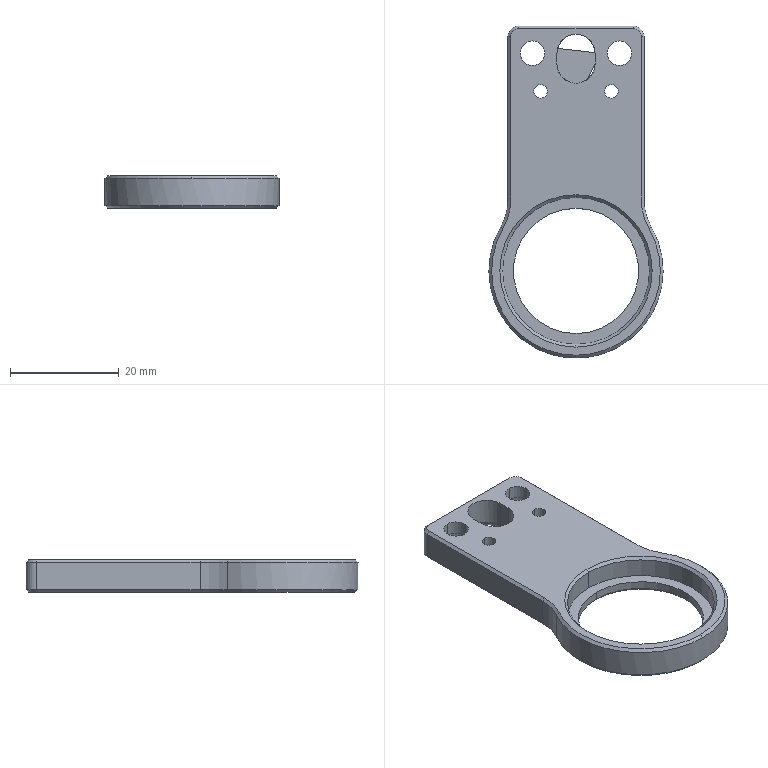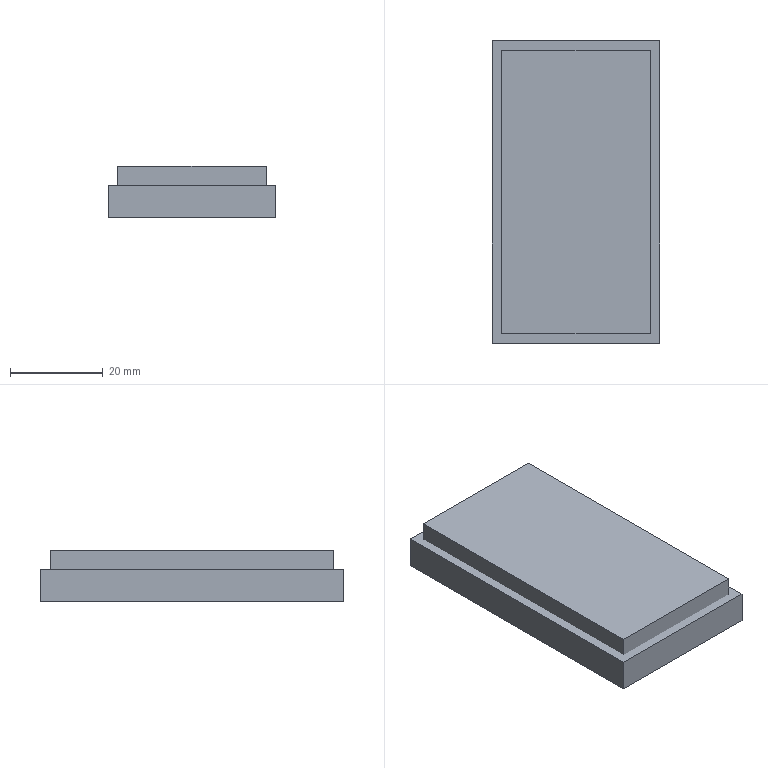CAM job | NX | 3-axis milling, drilling | part box 32 x 61 x 6 mm | stock box 36 x 65 x 11 mm
Tools:
number,name,description,diameter,corner_radius,flute_length,length,flutes
19,D80,Milling Tool-5 Parameters,80.0,0.0,50.0,75.0,2
15,D10,Milling Tool-5 Parameters,10.0,0.0,50.0,75.0,2
14,D10JING,Milling Tool-5 Parameters,10.0,0.0,50.0,75.0,2
1,D6A45,Milling Tool-5 Parameters,6.0,0.0,50.0,75.0,2
2,2.5ZT,Drilling Tool,2.5,0.0,35.0,50.0,2
8,4.5ZT,Drilling Tool,4.5,0.0,35.0,50.0,2
11,D4,Milling Tool-5 Parameters,4.0,0.0,50.0,75.0,2
18,D3R0.5,Milling Tool-5 Parameters,3.0,0.5,50.0,75.0,2
Operations:
program,operation,operation_type,tool,method,geometry_group,spindle_rpm,surface_speed,feed_per_tooth,feed_cut,feed_plunge,cut_length_mm,path_length_mm,cut_time_min,machine_time_min
1,FLOOR_WALL,VolumeBased25DMillingOperation,D80,METHOD,A,5000.0,1256.0,0.12,1200.0,100.0,157.0,211.0,0.1308,0.1362
1,ZLEVEL_PROFILE,ZLevelMilling,D10,METHOD,A,9500.0,298.0,0.1842,3500.0,1000.0,1623.323,1686.323,0.4976,0.5039
1,HOLE_MILLING_COPY,CylinderMilling,D10,METHOD,A,9500.0,0.0,0.0,2500.0,1000.0,340.477,404.477,0.1385,0.1449
1,HOLE_MILLING_COPY_COPY,CylinderMilling,D10,METHOD,A,9500.0,0.0,0.0,2500.0,1000.0,207.503,277.003,0.0854,0.0923
1,ZLEVEL_PROFILE_COPY,ZLevelMilling,D10JING,METHOD,A,9500.0,298.0,0.0789,1500.0,1000.0,297.363,451.982,0.2173,0.2328
1,SPOT_DRILLING,Operation,D6A45,METHOD,A,9500.0,179.0,0.0132,250.0,0.0,16.0,146.999,0.064,0.0771
1,DRILLING_COPY_COPY_COPY,Operation,2.5ZT,METHOD,A,2500.0,19.0,0.02,100.0,0.0,22.502,121.346,0.225,0.2349
1,DRILLING,Operation,4.5ZT,METHOD,A,2500.0,35.0,0.04,200.0,0.0,16.704,112.687,0.0835,0.0931
1,PLANAR_PROFILE,PlanarMilling,D6A45,METHOD,A,9500.0,179.0,0.0789,1500.0,500.0,334.467,824.513,0.2581,0.3071
1,刀补,CylinderMilling,D10,METHOD,A,9500.0,0.0,0.0789,1500.0,1000.0,181.868,245.868,0.1248,0.1312
2,FLOOR_WALL_COPY,VolumeBased25DMillingOperation,D80,METHOD,B,5000.0,1256.0,0.2,2000.0,100.0,785.0,1638.401,0.3925,0.4778
2,FLOOR_WALL_COPY_COPY,VolumeBased25DMillingOperation,D80,METHOD,B,5000.0,1256.0,0.12,1200.0,100.0,157.0,211.0,0.1308,0.1362
2,HOLE_MILLING_2,CylinderMilling,D4,METHOD,B,9500.0,119.0,0.0658,1250.0,100.0,216.94,358.94,0.1736,0.1878
2,ZLEVEL_PROFILE_COPY_1,ZLevelMilling,D4,METHOD,B,9500.0,119.0,0.1053,2000.0,1000.0,1006.015,1069.015,0.5192,0.5255
2,ZLEVEL_PROFILE_1,ZLevelMilling,D3R0.5,METHOD,B,9500.0,89.0,0.1316,2500.0,1000.0,4312.057,4507.039,1.729,1.748
2,PLANAR_PROFILE_COPY,PlanarMilling,D6A45,METHOD,B,9500.0,179.0,0.0789,1500.0,500.0,311.51,749.263,0.2388,0.2826